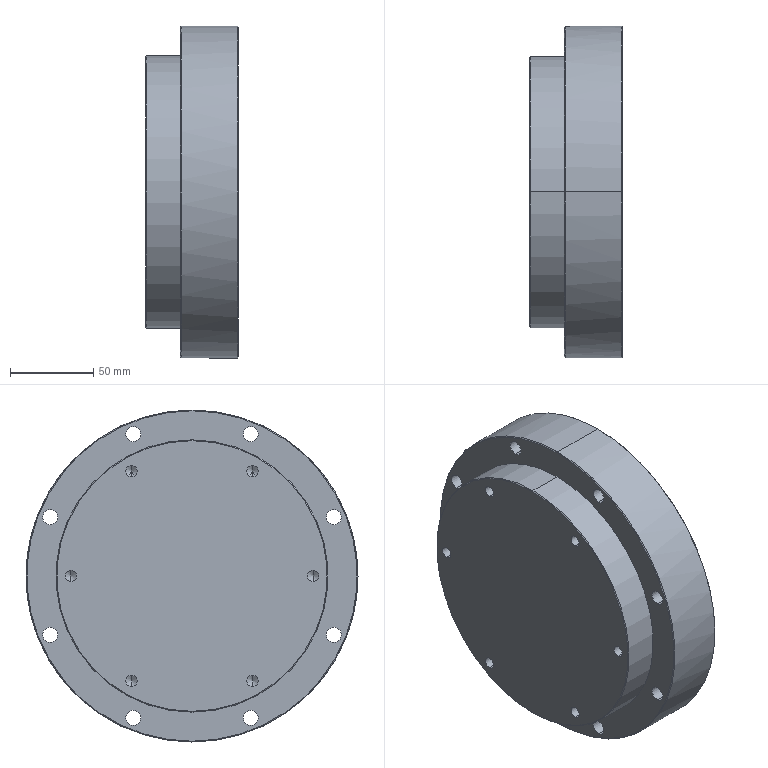Part | SolidWorks | features BaseBody 1 | 1 solid | 53 faces | box 56 x 200 x 200 mm | volume 1520895 mm3 | cylinder 32 | cone 18 | plane 3 | commonest cylinder face diameters 9 x16 6.8 x12 164 x2 200 x2
STEP:
#1=CARTESIAN_POINT('',(56.,85.459,-30.898));
#2=VERTEX_POINT('',#1);
#3=CARTESIAN_POINT('',(56.,85.459,-39.898));
#4=VERTEX_POINT('',#3);
#5=CARTESIAN_POINT('',(56.,85.459,-35.398));
#6=DIRECTION('',(1.,0.,0.));
#7=DIRECTION('',(0.,0.,1.));
#8=AXIS2_PLACEMENT_3D('',#5,#6,#7);
#9=CIRCLE('',#8,4.5);
#10=EDGE_CURVE('',#2,#4,#9,.T.);
#11=ORIENTED_EDGE('',*,*,#10,.T.);
#12=CARTESIAN_POINT('',(21.,85.459,-39.898));
#13=VERTEX_POINT('',#12);
#14=CARTESIAN_POINT('',(56.,85.459,-39.898));
#15=DIRECTION('',(-1.,0.,0.));
#16=VECTOR('',#15,1000.);
#17=LINE('',#14,#16);
#18=EDGE_CURVE('',#4,#13,#17,.T.);
#19=ORIENTED_EDGE('',*,*,#18,.T.);
#20=CARTESIAN_POINT('',(21.,85.459,-30.898));
#21=VERTEX_POINT('',#20);
#22=CARTESIAN_POINT('',(21.,85.459,-35.398));
#23=DIRECTION('',(1.,0.,0.));
#24=DIRECTION('',(0.,0.,1.));
#25=AXIS2_PLACEMENT_3D('',#22,#23,#24);
#26=CIRCLE('',#25,4.5);
#27=EDGE_CURVE('',#21,#13,#26,.T.);
#28=ORIENTED_EDGE('',*,*,#27,.F.);
#29=CARTESIAN_POINT('',(56.,85.459,-30.898));
#30=DIRECTION('',(-1.,0.,0.));
#31=VECTOR('',#30,1000.);
#32=LINE('',#29,#31);
#33=EDGE_CURVE('',#2,#21,#32,.T.);
#34=ORIENTED_EDGE('',*,*,#33,.F.);
#35=EDGE_LOOP('',(#11,#19,#28,#34));
#36=FACE_OUTER_BOUND('',#35,.T.);
#37=CARTESIAN_POINT('',(56.,85.459,-35.398));
#38=DIRECTION('',(-1.,0.,0.));
#39=DIRECTION('',(0.,0.,1.));
#40=AXIS2_PLACEMENT_3D('',#37,#38,#39);
#41=CYLINDRICAL_SURFACE('',#40,4.5);
#42=ADVANCED_FACE('',(#36),#41,.F.);
#43=CARTESIAN_POINT('',(56.,35.398,-80.959));
#44=VERTEX_POINT('',#43);
#45=CARTESIAN_POINT('',(56.,35.398,-89.959));
#46=VERTEX_POINT('',#45);
#47=CARTESIAN_POINT('',(56.,35.398,-85.459));
#48=DIRECTION('',(1.,0.,0.));
#49=DIRECTION('',(0.,0.,1.));
#50=AXIS2_PLACEMENT_3D('',#47,#48,#49);
#51=CIRCLE('',#50,4.5);
#52=EDGE_CURVE('',#44,#46,#51,.T.);
#53=ORIENTED_EDGE('',*,*,#52,.T.);
#54=CARTESIAN_POINT('',(21.,35.398,-89.959));
#55=VERTEX_POINT('',#54);
#56=CARTESIAN_POINT('',(56.,35.398,-89.959));
#57=DIRECTION('',(-1.,0.,0.));
#58=VECTOR('',#57,1000.);
#59=LINE('',#56,#58);
#60=EDGE_CURVE('',#46,#55,#59,.T.);
#61=ORIENTED_EDGE('',*,*,#60,.T.);
#62=CARTESIAN_POINT('',(21.,35.398,-80.959));
#63=VERTEX_POINT('',#62);
#64=CARTESIAN_POINT('',(21.,35.398,-85.459));
#65=DIRECTION('',(1.,0.,0.));
#66=DIRECTION('',(0.,0.,1.));
#67=AXIS2_PLACEMENT_3D('',#64,#65,#66);
#68=CIRCLE('',#67,4.5);
#69=EDGE_CURVE('',#63,#55,#68,.T.);
#70=ORIENTED_EDGE('',*,*,#69,.F.);
#71=CARTESIAN_POINT('',(56.,35.398,-80.959));
#72=DIRECTION('',(-1.,0.,0.));
#73=VECTOR('',#72,1000.);
#74=LINE('',#71,#73);
#75=EDGE_CURVE('',#44,#63,#74,.T.);
#76=ORIENTED_EDGE('',*,*,#75,.F.);
#77=EDGE_LOOP('',(#53,#61,#70,#76));
#78=FACE_OUTER_BOUND('',#77,.T.);
#79=CARTESIAN_POINT('',(56.,35.398,-85.459));
#80=DIRECTION('',(-1.,0.,0.));
#81=DIRECTION('',(0.,0.,1.));
#82=AXIS2_PLACEMENT_3D('',#79,#80,#81);
#83=CYLINDRICAL_SURFACE('',#82,4.5);
#84=ADVANCED_FACE('',(#78),#83,.F.);
#85=CARTESIAN_POINT('',(56.,-35.398,-80.959));
#86=VERTEX_POINT('',#85);
#87=CARTESIAN_POINT('',(56.,-35.398,-89.959));
#88=VERTEX_POINT('',#87);
#89=CARTESIAN_POINT('',(56.,-35.398,-85.459));
#90=DIRECTION('',(1.,0.,0.));
#91=DIRECTION('',(0.,0.,1.));
#92=AXIS2_PLACEMENT_3D('',#89,#90,#91);
#93=CIRCLE('',#92,4.5);
#94=EDGE_CURVE('',#86,#88,#93,.T.);
#95=ORIENTED_EDGE('',*,*,#94,.T.);
#96=CARTESIAN_POINT('',(21.,-35.398,-89.959));
#97=VERTEX_POINT('',#96);
#98=CARTESIAN_POINT('',(56.,-35.398,-89.959));
#99=DIRECTION('',(-1.,0.,0.));
#100=VECTOR('',#99,1000.);
#101=LINE('',#98,#100);
#102=EDGE_CURVE('',#88,#97,#101,.T.);
#103=ORIENTED_EDGE('',*,*,#102,.T.);
#104=CARTESIAN_POINT('',(21.,-35.398,-80.959));
#105=VERTEX_POINT('',#104);
#106=CARTESIAN_POINT('',(21.,-35.398,-85.459));
#107=DIRECTION('',(1.,0.,0.));
#108=DIRECTION('',(0.,0.,1.));
#109=AXIS2_PLACEMENT_3D('',#106,#107,#108);
#110=CIRCLE('',#109,4.5);
#111=EDGE_CURVE('',#105,#97,#110,.T.);
#112=ORIENTED_EDGE('',*,*,#111,.F.);
#113=CARTESIAN_POINT('',(56.,-35.398,-80.959));
#114=DIRECTION('',(-1.,0.,0.));
#115=VECTOR('',#114,1000.);
#116=LINE('',#113,#115);
#117=EDGE_CURVE('',#86,#105,#116,.T.);
#118=ORIENTED_EDGE('',*,*,#117,.F.);
#119=EDGE_LOOP('',(#95,#103,#112,#118));
#120=FACE_OUTER_BOUND('',#119,.T.);
#121=CARTESIAN_POINT('',(56.,-35.398,-85.459));
#122=DIRECTION('',(-1.,0.,0.));
#123=DIRECTION('',(0.,0.,1.));
#124=AXIS2_PLACEMENT_3D('',#121,#122,#123);
#125=CYLINDRICAL_SURFACE('',#124,4.5);
#126=ADVANCED_FACE('',(#120),#125,.F.);
#127=CARTESIAN_POINT('',(56.,-85.459,-30.898));
#128=VERTEX_POINT('',#127);
#129=CARTESIAN_POINT('',(56.,-85.459,-39.898));
#130=VERTEX_POINT('',#129);
#131=CARTESIAN_POINT('',(56.,-85.459,-35.398));
#132=DIRECTION('',(1.,0.,0.));
#133=DIRECTION('',(0.,0.,1.));
#134=AXIS2_PLACEMENT_3D('',#131,#132,#133);
#135=CIRCLE('',#134,4.5);
#136=EDGE_CURVE('',#128,#130,#135,.T.);
#137=ORIENTED_EDGE('',*,*,#136,.T.);
#138=CARTESIAN_POINT('',(21.,-85.459,-39.898));
#139=VERTEX_POINT('',#138);
#140=CARTESIAN_POINT('',(56.,-85.459,-39.898));
#141=DIRECTION('',(-1.,0.,0.));
#142=VECTOR('',#141,1000.);
#143=LINE('',#140,#142);
#144=EDGE_CURVE('',#130,#139,#143,.T.);
#145=ORIENTED_EDGE('',*,*,#144,.T.);
#146=CARTESIAN_POINT('',(21.,-85.459,-30.898));
#147=VERTEX_POINT('',#146);
#148=CARTESIAN_POINT('',(21.,-85.459,-35.398));
#149=DIRECTION('',(1.,0.,0.));
#150=DIRECTION('',(0.,0.,1.));
#151=AXIS2_PLACEMENT_3D('',#148,#149,#150);
#152=CIRCLE('',#151,4.5);
#153=EDGE_CURVE('',#147,#139,#152,.T.);
#154=ORIENTED_EDGE('',*,*,#153,.F.);
#155=CARTESIAN_POINT('',(56.,-85.459,-30.898));
#156=DIRECTION('',(-1.,0.,0.));
#157=VECTOR('',#156,1000.);
#158=LINE('',#155,#157);
#159=EDGE_CURVE('',#128,#147,#158,.T.);
#160=ORIENTED_EDGE('',*,*,#159,.F.);
#161=EDGE_LOOP('',(#137,#145,#154,#160));
#162=FACE_OUTER_BOUND('',#161,.T.);
#163=CARTESIAN_POINT('',(56.,-85.459,-35.398));
#164=DIRECTION('',(-1.,0.,0.));
#165=DIRECTION('',(0.,0.,1.));
#166=AXIS2_PLACEMENT_3D('',#163,#164,#165);
#167=CYLINDRICAL_SURFACE('',#166,4.5);
#168=ADVANCED_FACE('',(#162),#167,.F.);
#169=CARTESIAN_POINT('',(56.,-85.459,39.898));
#170=VERTEX_POINT('',#169);
#171=CARTESIAN_POINT('',(56.,-85.459,30.898));
#172=VERTEX_POINT('',#171);
#173=CARTESIAN_POINT('',(56.,-85.459,35.398));
#174=DIRECTION('',(1.,0.,0.));
#175=DIRECTION('',(0.,0.,1.));
#176=AXIS2_PLACEMENT_3D('',#173,#174,#175);
#177=CIRCLE('',#176,4.5);
#178=EDGE_CURVE('',#170,#172,#177,.T.);
#179=ORIENTED_EDGE('',*,*,#178,.T.);
#180=CARTESIAN_POINT('',(21.,-85.459,30.898));
#181=VERTEX_POINT('',#180);
#182=CARTESIAN_POINT('',(56.,-85.459,30.898));
#183=DIRECTION('',(-1.,0.,0.));
#184=VECTOR('',#183,1000.);
#185=LINE('',#182,#184);
#186=EDGE_CURVE('',#172,#181,#185,.T.);
#187=ORIENTED_EDGE('',*,*,#186,.T.);
#188=CARTESIAN_POINT('',(21.,-85.459,39.898));
#189=VERTEX_POINT('',#188);
#190=CARTESIAN_POINT('',(21.,-85.459,35.398));
#191=DIRECTION('',(1.,0.,0.));
#192=DIRECTION('',(0.,0.,1.));
#193=AXIS2_PLACEMENT_3D('',#190,#191,#192);
#194=CIRCLE('',#193,4.5);
#195=EDGE_CURVE('',#189,#181,#194,.T.);
#196=ORIENTED_EDGE('',*,*,#195,.F.);
#197=CARTESIAN_POINT('',(56.,-85.459,39.898));
#198=DIRECTION('',(-1.,0.,0.));
#199=VECTOR('',#198,1000.);
#200=LINE('',#197,#199);
#201=EDGE_CURVE('',#170,#189,#200,.T.);
#202=ORIENTED_EDGE('',*,*,#201,.F.);
#203=EDGE_LOOP('',(#179,#187,#196,#202));
#204=FACE_OUTER_BOUND('',#203,.T.);
#205=CARTESIAN_POINT('',(56.,-85.459,35.398));
#206=DIRECTION('',(-1.,0.,0.));
#207=DIRECTION('',(0.,0.,1.));
#208=AXIS2_PLACEMENT_3D('',#205,#206,#207);
#209=CYLINDRICAL_SURFACE('',#208,4.5);
#210=ADVANCED_FACE('',(#204),#209,.F.);
#211=CARTESIAN_POINT('',(56.,-35.398,89.959));
#212=VERTEX_POINT('',#211);
#213=CARTESIAN_POINT('',(56.,-35.398,80.959));
#214=VERTEX_POINT('',#213);
#215=CARTESIAN_POINT('',(56.,-35.398,85.459));
#216=DIRECTION('',(1.,0.,0.));
#217=DIRECTION('',(0.,0.,1.));
#218=AXIS2_PLACEMENT_3D('',#215,#216,#217);
#219=CIRCLE('',#218,4.5);
#220=EDGE_CURVE('',#212,#214,#219,.T.);
#221=ORIENTED_EDGE('',*,*,#220,.T.);
#222=CARTESIAN_POINT('',(21.,-35.398,80.959));
#223=VERTEX_POINT('',#222);
#224=CARTESIAN_POINT('',(56.,-35.398,80.959));
#225=DIRECTION('',(-1.,0.,0.));
#226=VECTOR('',#225,1000.);
#227=LINE('',#224,#226);
#228=EDGE_CURVE('',#214,#223,#227,.T.);
#229=ORIENTED_EDGE('',*,*,#228,.T.);
#230=CARTESIAN_POINT('',(21.,-35.398,89.959));
#231=VERTEX_POINT('',#230);
#232=CARTESIAN_POINT('',(21.,-35.398,85.459));
#233=DIRECTION('',(1.,0.,0.));
#234=DIRECTION('',(0.,0.,1.));
#235=AXIS2_PLACEMENT_3D('',#232,#233,#234);
#236=CIRCLE('',#235,4.5);
#237=EDGE_CURVE('',#231,#223,#236,.T.);
#238=ORIENTED_EDGE('',*,*,#237,.F.);
#239=CARTESIAN_POINT('',(56.,-35.398,89.959));
#240=DIRECTION('',(-1.,0.,0.));
#241=VECTOR('',#240,1000.);
#242=LINE('',#239,#241);
#243=EDGE_CURVE('',#212,#231,#242,.T.);
#244=ORIENTED_EDGE('',*,*,#243,.F.);
#245=EDGE_LOOP('',(#221,#229,#238,#244));
#246=FACE_OUTER_BOUND('',#245,.T.);
#247=CARTESIAN_POINT('',(56.,-35.398,85.459));
#248=DIRECTION('',(-1.,0.,0.));
#249=DIRECTION('',(0.,0.,1.));
#250=AXIS2_PLACEMENT_3D('',#247,#248,#249);
#251=CYLINDRICAL_SURFACE('',#250,4.5);
#252=ADVANCED_FACE('',(#246),#251,.F.);
#253=CARTESIAN_POINT('',(56.,35.398,89.959));
#254=VERTEX_POINT('',#253);
#255=CARTESIAN_POINT('',(56.,35.398,80.959));
#256=VERTEX_POINT('',#255);
#257=CARTESIAN_POINT('',(56.,35.398,85.459));
#258=DIRECTION('',(1.,0.,0.));
#259=DIRECTION('',(0.,0.,1.));
#260=AXIS2_PLACEMENT_3D('',#257,#258,#259);
#261=CIRCLE('',#260,4.5);
#262=EDGE_CURVE('',#254,#256,#261,.T.);
#263=ORIENTED_EDGE('',*,*,#262,.T.);
#264=CARTESIAN_POINT('',(21.,35.398,80.959));
#265=VERTEX_POINT('',#264);
#266=CARTESIAN_POINT('',(56.,35.398,80.959));
#267=DIRECTION('',(-1.,0.,0.));
#268=VECTOR('',#267,1000.);
#269=LINE('',#266,#268);
#270=EDGE_CURVE('',#256,#265,#269,.T.);
#271=ORIENTED_EDGE('',*,*,#270,.T.);
#272=CARTESIAN_POINT('',(21.,35.398,89.959));
#273=VERTEX_POINT('',#272);
#274=CARTESIAN_POINT('',(21.,35.398,85.459));
#275=DIRECTION('',(1.,0.,0.));
#276=DIRECTION('',(0.,0.,1.));
#277=AXIS2_PLACEMENT_3D('',#274,#275,#276);
#278=CIRCLE('',#277,4.5);
#279=EDGE_CURVE('',#273,#265,#278,.T.);
#280=ORIENTED_EDGE('',*,*,#279,.F.);
#281=CARTESIAN_POINT('',(56.,35.398,89.959));
#282=DIRECTION('',(-1.,0.,0.));
#283=VECTOR('',#282,1000.);
#284=LINE('',#281,#283);
#285=EDGE_CURVE('',#254,#273,#284,.T.);
#286=ORIENTED_EDGE('',*,*,#285,.F.);
#287=EDGE_LOOP('',(#263,#271,#280,#286));
#288=FACE_OUTER_BOUND('',#287,.T.);
#289=CARTESIAN_POINT('',(56.,35.398,85.459));
#290=DIRECTION('',(-1.,0.,0.));
#291=DIRECTION('',(0.,0.,1.));
#292=AXIS2_PLACEMENT_3D('',#289,#290,#291);
#293=CYLINDRICAL_SURFACE('',#292,4.5);
#294=ADVANCED_FACE('',(#288),#293,.F.);
#295=CARTESIAN_POINT('',(56.,85.459,39.898));
#296=VERTEX_POINT('',#295);
#297=CARTESIAN_POINT('',(56.,85.459,30.898));
#298=VERTEX_POINT('',#297);
#299=CARTESIAN_POINT('',(56.,85.459,35.398));
#300=DIRECTION('',(1.,0.,0.));
#301=DIRECTION('',(0.,0.,1.));
#302=AXIS2_PLACEMENT_3D('',#299,#300,#301);
#303=CIRCLE('',#302,4.5);
#304=EDGE_CURVE('',#296,#298,#303,.T.);
#305=ORIENTED_EDGE('',*,*,#304,.T.);
#306=CARTESIAN_POINT('',(21.,85.459,30.898));
#307=VERTEX_POINT('',#306);
#308=CARTESIAN_POINT('',(56.,85.459,30.898));
#309=DIRECTION('',(-1.,0.,0.));
#310=VECTOR('',#309,1000.);
#311=LINE('',#308,#310);
#312=EDGE_CURVE('',#298,#307,#311,.T.);
#313=ORIENTED_EDGE('',*,*,#312,.T.);
#314=CARTESIAN_POINT('',(21.,85.459,39.898));
#315=VERTEX_POINT('',#314);
#316=CARTESIAN_POINT('',(21.,85.459,35.398));
#317=DIRECTION('',(1.,0.,0.));
#318=DIRECTION('',(0.,0.,1.));
#319=AXIS2_PLACEMENT_3D('',#316,#317,#318);
#320=CIRCLE('',#319,4.5);
#321=EDGE_CURVE('',#315,#307,#320,.T.);
#322=ORIENTED_EDGE('',*,*,#321,.F.);
#323=CARTESIAN_POINT('',(56.,85.459,39.898));
#324=DIRECTION('',(-1.,0.,0.));
#325=VECTOR('',#324,1000.);
#326=LINE('',#323,#325);
#327=EDGE_CURVE('',#296,#315,#326,.T.);
#328=ORIENTED_EDGE('',*,*,#327,.F.);
#329=EDGE_LOOP('',(#305,#313,#322,#328));
#330=FACE_OUTER_BOUND('',#329,.T.);
#331=CARTESIAN_POINT('',(56.,85.459,35.398));
#332=DIRECTION('',(-1.,0.,0.));
#333=DIRECTION('',(0.,0.,1.));
#334=AXIS2_PLACEMENT_3D('',#331,#332,#333);
#335=CYLINDRICAL_SURFACE('',#334,4.5);
#336=ADVANCED_FACE('',(#330),#335,.F.);
#337=CARTESIAN_POINT('',(56.,-99.5,0.));
#338=VERTEX_POINT('',#337);
#339=CARTESIAN_POINT('',(56.,99.5,0.));
#340=VERTEX_POINT('',#339);
#341=CARTESIAN_POINT('',(56.,0.,0.));
#342=DIRECTION('',(-1.,0.,0.));
#343=DIRECTION('',(0.,-1.,0.));
#344=AXIS2_PLACEMENT_3D('',#341,#342,#343);
#345=CIRCLE('',#344,99.5);
#346=EDGE_CURVE('',#338,#340,#345,.T.);
#347=ORIENTED_EDGE('',*,*,#346,.T.);
#348=CARTESIAN_POINT('',(55.5,100.,0.));
#349=VERTEX_POINT('',#348);
#350=CARTESIAN_POINT('',(55.5,100.,0.));
#351=DIRECTION('',(-0.7071,0.7071,0.));
#352=VECTOR('',#351,1000.);
#353=LINE('',#350,#352);
#354=EDGE_CURVE('',#340,#349,#353,.T.);
#355=ORIENTED_EDGE('',*,*,#354,.T.);
#356=CARTESIAN_POINT('',(55.5,0.,100.));
#357=VERTEX_POINT('',#356);
#358=CARTESIAN_POINT('',(55.5,0.,0.));
#359=DIRECTION('',(1.,0.,0.));
#360=DIRECTION('',(0.,0.,1.));
#361=AXIS2_PLACEMENT_3D('',#358,#359,#360);
#362=CIRCLE('',#361,100.);
#363=EDGE_CURVE('',#349,#357,#362,.T.);
#364=ORIENTED_EDGE('',*,*,#363,.T.);
#365=CARTESIAN_POINT('',(55.5,-100.,0.));
#366=VERTEX_POINT('',#365);
#367=CARTESIAN_POINT('',(55.5,0.,0.));
#368=DIRECTION('',(1.,0.,0.));
#369=DIRECTION('',(0.,0.,1.));
#370=AXIS2_PLACEMENT_3D('',#367,#368,#369);
#371=CIRCLE('',#370,100.);
#372=EDGE_CURVE('',#357,#366,#371,.T.);
#373=ORIENTED_EDGE('',*,*,#372,.T.);
#374=CARTESIAN_POINT('',(55.5,-100.,0.));
#375=DIRECTION('',(-0.7071,-0.7071,0.));
#376=VECTOR('',#375,1000.);
#377=LINE('',#374,#376);
#378=EDGE_CURVE('',#338,#366,#377,.T.);
#379=ORIENTED_EDGE('',*,*,#378,.F.);
#380=EDGE_LOOP('',(#347,#355,#364,#373,#379));
#381=FACE_OUTER_BOUND('',#380,.T.);
#382=CARTESIAN_POINT('',(55.5,0.,0.));
#383=DIRECTION('',(-1.,0.,0.));
#384=DIRECTION('',(0.,-1.,0.));
#385=AXIS2_PLACEMENT_3D('',#382,#383,#384);
#386=CONICAL_SURFACE('',#385,100.,0.7854);
#387=ADVANCED_FACE('',(#381),#386,.T.);
#388=CARTESIAN_POINT('',(55.5,0.,-100.));
#389=VERTEX_POINT('',#388);
#390=CARTESIAN_POINT('',(55.5,0.,0.));
#391=DIRECTION('',(1.,0.,0.));
#392=DIRECTION('',(0.,0.,1.));
#393=AXIS2_PLACEMENT_3D('',#390,#391,#392);
#394=CIRCLE('',#393,100.);
#395=EDGE_CURVE('',#389,#349,#394,.T.);
#396=ORIENTED_EDGE('',*,*,#395,.F.);
#397=CARTESIAN_POINT('',(21.5,0.,-100.));
#398=VERTEX_POINT('',#397);
#399=CARTESIAN_POINT('',(0.,0.,-100.));
#400=DIRECTION('',(-1.,0.,0.));
#401=VECTOR('',#400,1000.);
#402=LINE('',#399,#401);
#403=EDGE_CURVE('',#389,#398,#402,.T.);
#404=ORIENTED_EDGE('',*,*,#403,.T.);
#405=CARTESIAN_POINT('',(21.5,0.,100.));
#406=VERTEX_POINT('',#405);
#407=CARTESIAN_POINT('',(21.5,0.,0.));
#408=DIRECTION('',(1.,0.,0.));
#409=DIRECTION('',(0.,0.,1.));
#410=AXIS2_PLACEMENT_3D('',#407,#408,#409);
#411=CIRCLE('',#410,100.);
#412=EDGE_CURVE('',#398,#406,#411,.T.);
#413=ORIENTED_EDGE('',*,*,#412,.T.);
#414=CARTESIAN_POINT('',(0.,0.,100.));
#415=DIRECTION('',(-1.,0.,0.));
#416=VECTOR('',#415,1000.);
#417=LINE('',#414,#416);
#418=EDGE_CURVE('',#357,#406,#417,.T.);
#419=ORIENTED_EDGE('',*,*,#418,.F.);
#420=ORIENTED_EDGE('',*,*,#363,.F.);
#421=EDGE_LOOP('',(#396,#404,#413,#419,#420));
#422=FACE_OUTER_BOUND('',#421,.T.);
#423=CARTESIAN_POINT('',(0.,0.,0.));
#424=DIRECTION('',(-1.,0.,0.));
#425=DIRECTION('',(0.,0.,1.));
#426=AXIS2_PLACEMENT_3D('',#423,#424,#425);
#427=CYLINDRICAL_SURFACE('',#426,100.);
#428=ADVANCED_FACE('',(#422),#427,.T.);
#429=CARTESIAN_POINT('',(21.,0.,82.));
#430=VERTEX_POINT('',#429);
#431=CARTESIAN_POINT('',(21.,0.,-82.));
#432=VERTEX_POINT('',#431);
#433=CARTESIAN_POINT('',(21.,0.,0.));
#434=DIRECTION('',(-1.,0.,0.));
#435=DIRECTION('',(0.,0.,1.));
#436=AXIS2_PLACEMENT_3D('',#433,#434,#435);
#437=CIRCLE('',#436,82.);
#438=EDGE_CURVE('',#430,#432,#437,.T.);
#439=ORIENTED_EDGE('',*,*,#438,.T.);
#440=CARTESIAN_POINT('',(0.5,0.,-82.));
#441=VERTEX_POINT('',#440);
#442=CARTESIAN_POINT('',(0.,0.,-82.));
#443=DIRECTION('',(-1.,0.,0.));
#444=VECTOR('',#443,1000.);
#445=LINE('',#442,#444);
#446=EDGE_CURVE('',#432,#441,#445,.T.);
#447=ORIENTED_EDGE('',*,*,#446,.T.);
#448=CARTESIAN_POINT('',(0.5,0.,82.));
#449=VERTEX_POINT('',#448);
#450=CARTESIAN_POINT('',(0.5,0.,0.));
#451=DIRECTION('',(1.,0.,0.));
#452=DIRECTION('',(0.,0.,1.));
#453=AXIS2_PLACEMENT_3D('',#450,#451,#452);
#454=CIRCLE('',#453,82.);
#455=EDGE_CURVE('',#441,#449,#454,.T.);
#456=ORIENTED_EDGE('',*,*,#455,.T.);
#457=CARTESIAN_POINT('',(0.,0.,82.));
#458=DIRECTION('',(-1.,0.,0.));
#459=VECTOR('',#458,1000.);
#460=LINE('',#457,#459);
#461=EDGE_CURVE('',#430,#449,#460,.T.);
#462=ORIENTED_EDGE('',*,*,#461,.F.);
#463=EDGE_LOOP('',(#439,#447,#456,#462));
#464=FACE_OUTER_BOUND('',#463,.T.);
#465=CARTESIAN_POINT('',(0.,0.,0.));
#466=DIRECTION('',(-1.,0.,0.));
#467=DIRECTION('',(0.,0.,1.));
#468=AXIS2_PLACEMENT_3D('',#465,#466,#467);
#469=CYLINDRICAL_SURFACE('',#468,82.);
#470=ADVANCED_FACE('',(#464),#469,.T.);
#471=CARTESIAN_POINT('',(21.,0.,-99.5));
#472=VERTEX_POINT('',#471);
#473=CARTESIAN_POINT('',(21.,0.,99.5));
#474=VERTEX_POINT('',#473);
#475=CARTESIAN_POINT('',(21.,0.,0.));
#476=DIRECTION('',(1.,0.,0.));
#477=DIRECTION('',(0.,0.,-1.));
#478=AXIS2_PLACEMENT_3D('',#475,#476,#477);
#479=CIRCLE('',#478,99.5);
#480=EDGE_CURVE('',#472,#474,#479,.T.);
#481=ORIENTED_EDGE('',*,*,#480,.T.);
#482=CARTESIAN_POINT('',(21.5,0.,100.));
#483=DIRECTION('',(0.7071,0.,0.7071));
#484=VECTOR('',#483,1000.);
#485=LINE('',#482,#484);
#486=EDGE_CURVE('',#474,#406,#485,.T.);
#487=ORIENTED_EDGE('',*,*,#486,.T.);
#488=ORIENTED_EDGE('',*,*,#412,.F.);
#489=CARTESIAN_POINT('',(21.5,0.,-100.));
#490=DIRECTION('',(0.7071,0.,-0.7071));
#491=VECTOR('',#490,1000.);
#492=LINE('',#489,#491);
#493=EDGE_CURVE('',#472,#398,#492,.T.);
#494=ORIENTED_EDGE('',*,*,#493,.F.);
#495=EDGE_LOOP('',(#481,#487,#488,#494));
#496=FACE_OUTER_BOUND('',#495,.T.);
#497=CARTESIAN_POINT('',(21.5,0.,0.));
#498=DIRECTION('',(1.,0.,0.));
#499=DIRECTION('',(0.,0.,-1.));
#500=AXIS2_PLACEMENT_3D('',#497,#498,#499);
#501=CONICAL_SURFACE('',#500,100.,0.7854);
#502=ADVANCED_FACE('',(#496),#501,.T.);
#503=CARTESIAN_POINT('',(0.,0.,-81.5));
#504=VERTEX_POINT('',#503);
#505=CARTESIAN_POINT('',(0.,0.,81.5));
#506=VERTEX_POINT('',#505);
#507=CARTESIAN_POINT('',(0.,0.,0.));
#508=DIRECTION('',(1.,0.,0.));
#509=DIRECTION('',(0.,0.,-1.));
#510=AXIS2_PLACEMENT_3D('',#507,#508,#509);
#511=CIRCLE('',#510,81.5);
#512=EDGE_CURVE('',#504,#506,#511,.T.);
#513=ORIENTED_EDGE('',*,*,#512,.T.);
#514=CARTESIAN_POINT('',(0.5,0.,82.));
#515=DIRECTION('',(0.7071,0.,0.7071));
#516=VECTOR('',#515,1000.);
#517=LINE('',#514,#516);
#518=EDGE_CURVE('',#506,#449,#517,.T.);
#519=ORIENTED_EDGE('',*,*,#518,.T.);
#520=ORIENTED_EDGE('',*,*,#455,.F.);
#521=CARTESIAN_POINT('',(0.5,0.,-82.));
#522=DIRECTION('',(0.7071,0.,-0.7071));
#523=VECTOR('',#522,1000.);
#524=LINE('',#521,#523);
#525=EDGE_CURVE('',#504,#441,#524,.T.);
#526=ORIENTED_EDGE('',*,*,#525,.F.);
#527=EDGE_LOOP('',(#513,#519,#520,#526));
#528=FACE_OUTER_BOUND('',#527,.T.);
#529=CARTESIAN_POINT('',(0.5,0.,0.));
#530=DIRECTION('',(1.,0.,0.));
#531=DIRECTION('',(0.,0.,-1.));
#532=AXIS2_PLACEMENT_3D('',#529,#530,#531);
#533=CONICAL_SURFACE('',#532,82.,0.7854);
#534=ADVANCED_FACE('',(#528),#533,.T.);
#535=CARTESIAN_POINT('',(18.75,73.,-3.4));
#536=VERTEX_POINT('',#535);
#537=CARTESIAN_POINT('',(18.75,73.,3.4));
#538=VERTEX_POINT('',#537);
#539=CARTESIAN_POINT('',(18.75,73.,0.));
#540=DIRECTION('',(-1.,0.,0.));
#541=DIRECTION('',(0.,0.,1.));
#542=AXIS2_PLACEMENT_3D('',#539,#540,#541);
#543=CIRCLE('',#542,3.4);
#544=EDGE_CURVE('',#536,#538,#543,.T.);
#545=ORIENTED_EDGE('',*,*,#544,.F.);
#546=CARTESIAN_POINT('',(0.,73.,-3.4));
#547=VERTEX_POINT('',#546);
#548=CARTESIAN_POINT('',(0.,73.,-3.4));
#549=DIRECTION('',(-1.,0.,0.));
#550=VECTOR('',#549,1000.);
#551=LINE('',#548,#550);
#552=EDGE_CURVE('',#536,#547,#551,.T.);
#553=ORIENTED_EDGE('',*,*,#552,.T.);
#554=CARTESIAN_POINT('',(0.,73.,3.4));
#555=VERTEX_POINT('',#554);
#556=CARTESIAN_POINT('',(0.,73.,0.));
#557=DIRECTION('',(-1.,0.,0.));
#558=DIRECTION('',(0.,0.,1.));
#559=AXIS2_PLACEMENT_3D('',#556,#557,#558);
#560=CIRCLE('',#559,3.4);
#561=EDGE_CURVE('',#547,#555,#560,.T.);
#562=ORIENTED_EDGE('',*,*,#561,.T.);
#563=CARTESIAN_POINT('',(0.,73.,3.4));
#564=DIRECTION('',(-1.,0.,0.));
#565=VECTOR('',#564,1000.);
#566=LINE('',#563,#565);
#567=EDGE_CURVE('',#538,#555,#566,.T.);
#568=ORIENTED_EDGE('',*,*,#567,.F.);
#569=EDGE_LOOP('',(#545,#553,#562,#568));
#570=FACE_OUTER_BOUND('',#569,.T.);
#571=CARTESIAN_POINT('',(0.,73.,0.));
#572=DIRECTION('',(-1.,0.,0.));
#573=DIRECTION('',(0.,0.,1.));
#574=AXIS2_PLACEMENT_3D('',#571,#572,#573);
#575=CYLINDRICAL_SURFACE('',#574,3.4);
#576=ADVANCED_FACE('',(#570),#575,.F.);
#577=CARTESIAN_POINT('',(18.75,36.5,-66.62));
#578=VERTEX_POINT('',#577);
#579=CARTESIAN_POINT('',(18.75,36.5,-59.82));
#580=VERTEX_POINT('',#579);
#581=CARTESIAN_POINT('',(18.75,36.5,-63.22));
#582=DIRECTION('',(-1.,0.,0.));
#583=DIRECTION('',(0.,0.,1.));
#584=AXIS2_PLACEMENT_3D('',#581,#582,#583);
#585=CIRCLE('',#584,3.4);
#586=EDGE_CURVE('',#578,#580,#585,.T.);
#587=ORIENTED_EDGE('',*,*,#586,.F.);
#588=CARTESIAN_POINT('',(0.,36.5,-66.62));
#589=VERTEX_POINT('',#588);
#590=CARTESIAN_POINT('',(0.,36.5,-66.62));
#591=DIRECTION('',(-1.,0.,0.));
#592=VECTOR('',#591,1000.);
#593=LINE('',#590,#592);
#594=EDGE_CURVE('',#578,#589,#593,.T.);
#595=ORIENTED_EDGE('',*,*,#594,.T.);
#596=CARTESIAN_POINT('',(0.,36.5,-59.82));
#597=VERTEX_POINT('',#596);
#598=CARTESIAN_POINT('',(0.,36.5,-63.22));
#599=DIRECTION('',(-1.,0.,0.));
#600=DIRECTION('',(0.,0.,1.));
#601=AXIS2_PLACEMENT_3D('',#598,#599,#600);
#602=CIRCLE('',#601,3.4);
#603=EDGE_CURVE('',#589,#597,#602,.T.);
#604=ORIENTED_EDGE('',*,*,#603,.T.);
#605=CARTESIAN_POINT('',(0.,36.5,-59.82));
#606=DIRECTION('',(-1.,0.,0.));
#607=VECTOR('',#606,1000.);
#608=LINE('',#605,#607);
#609=EDGE_CURVE('',#580,#597,#608,.T.);
#610=ORIENTED_EDGE('',*,*,#609,.F.);
#611=EDGE_LOOP('',(#587,#595,#604,#610));
#612=FACE_OUTER_BOUND('',#611,.T.);
#613=CARTESIAN_POINT('',(0.,36.5,-63.22));
#614=DIRECTION('',(-1.,0.,0.));
#615=DIRECTION('',(0.,0.,1.));
#616=AXIS2_PLACEMENT_3D('',#613,#614,#615);
#617=CYLINDRICAL_SURFACE('',#616,3.4);
#618=ADVANCED_FACE('',(#612),#617,.F.);
#619=CARTESIAN_POINT('',(18.75,-36.5,-66.62));
#620=VERTEX_POINT('',#619);
#621=CARTESIAN_POINT('',(18.75,-36.5,-59.82));
#622=VERTEX_POINT('',#621);
#623=CARTESIAN_POINT('',(18.75,-36.5,-63.22));
#624=DIRECTION('',(-1.,0.,0.));
#625=DIRECTION('',(0.,0.,1.));
#626=AXIS2_PLACEMENT_3D('',#623,#624,#625);
#627=CIRCLE('',#626,3.4);
#628=EDGE_CURVE('',#620,#622,#627,.T.);
#629=ORIENTED_EDGE('',*,*,#628,.F.);
#630=CARTESIAN_POINT('',(0.,-36.5,-66.62));
#631=VERTEX_POINT('',#630);
#632=CARTESIAN_POINT('',(0.,-36.5,-66.62));
#633=DIRECTION('',(-1.,0.,0.));
#634=VECTOR('',#633,1000.);
#635=LINE('',#632,#634);
#636=EDGE_CURVE('',#620,#631,#635,.T.);
#637=ORIENTED_EDGE('',*,*,#636,.T.);
#638=CARTESIAN_POINT('',(0.,-36.5,-59.82));
#639=VERTEX_POINT('',#638);
#640=CARTESIAN_POINT('',(0.,-36.5,-63.22));
#641=DIRECTION('',(-1.,0.,0.));
#642=DIRECTION('',(0.,0.,1.));
#643=AXIS2_PLACEMENT_3D('',#640,#641,#642);
#644=CIRCLE('',#643,3.4);
#645=EDGE_CURVE('',#631,#639,#644,.T.);
#646=ORIENTED_EDGE('',*,*,#645,.T.);
#647=CARTESIAN_POINT('',(0.,-36.5,-59.82));
#648=DIRECTION('',(-1.,0.,0.));
#649=VECTOR('',#648,1000.);
#650=LINE('',#647,#649);
#651=EDGE_CURVE('',#622,#639,#650,.T.);
#652=ORIENTED_EDGE('',*,*,#651,.F.);
#653=EDGE_LOOP('',(#629,#637,#646,#652));
#654=FACE_OUTER_BOUND('',#653,.T.);
#655=CARTESIAN_POINT('',(0.,-36.5,-63.22));
#656=DIRECTION('',(-1.,0.,0.));
#657=DIRECTION('',(0.,0.,1.));
#658=AXIS2_PLACEMENT_3D('',#655,#656,#657);
#659=CYLINDRICAL_SURFACE('',#658,3.4);
#660=ADVANCED_FACE('',(#654),#659,.F.);
#661=CARTESIAN_POINT('',(18.75,-73.,-3.4));
#662=VERTEX_POINT('',#661);
#663=CARTESIAN_POINT('',(18.75,-73.,3.4));
#664=VERTEX_POINT('',#663);
#665=CARTESIAN_POINT('',(18.75,-73.,0.));
#666=DIRECTION('',(-1.,0.,0.));
#667=DIRECTION('',(0.,0.,1.));
#668=AXIS2_PLACEMENT_3D('',#665,#666,#667);
#669=CIRCLE('',#668,3.4);
#670=EDGE_CURVE('',#662,#664,#669,.T.);
#671=ORIENTED_EDGE('',*,*,#670,.F.);
#672=CARTESIAN_POINT('',(0.,-73.,-3.4));
#673=VERTEX_POINT('',#672);
#674=CARTESIAN_POINT('',(0.,-73.,-3.4));
#675=DIRECTION('',(-1.,0.,0.));
#676=VECTOR('',#675,1000.);
#677=LINE('',#674,#676);
#678=EDGE_CURVE('',#662,#673,#677,.T.);
#679=ORIENTED_EDGE('',*,*,#678,.T.);
#680=CARTESIAN_POINT('',(0.,-73.,3.4));
#681=VERTEX_POINT('',#680);
#682=CARTESIAN_POINT('',(0.,-73.,0.));
#683=DIRECTION('',(-1.,0.,0.));
#684=DIRECTION('',(0.,0.,1.));
#685=AXIS2_PLACEMENT_3D('',#682,#683,#684);
#686=CIRCLE('',#685,3.4);
#687=EDGE_CURVE('',#673,#681,#686,.T.);
#688=ORIENTED_EDGE('',*,*,#687,.T.);
#689=CARTESIAN_POINT('',(0.,-73.,3.4));
#690=DIRECTION('',(-1.,0.,0.));
#691=VECTOR('',#690,1000.);
#692=LINE('',#689,#691);
#693=EDGE_CURVE('',#664,#681,#692,.T.);
#694=ORIENTED_EDGE('',*,*,#693,.F.);
#695=EDGE_LOOP('',(#671,#679,#688,#694));
#696=FACE_OUTER_BOUND('',#695,.T.);
#697=CARTESIAN_POINT('',(0.,-73.,0.));
#698=DIRECTION('',(-1.,0.,0.));
#699=DIRECTION('',(0.,0.,1.));
#700=AXIS2_PLACEMENT_3D('',#697,#698,#699);
#701=CYLINDRICAL_SURFACE('',#700,3.4);
#702=ADVANCED_FACE('',(#696),#701,.F.);
#703=CARTESIAN_POINT('',(18.75,-36.5,59.82));
#704=VERTEX_POINT('',#703);
#705=CARTESIAN_POINT('',(18.75,-36.5,66.62));
#706=VERTEX_POINT('',#705);
#707=CARTESIAN_POINT('',(18.75,-36.5,63.22));
#708=DIRECTION('',(-1.,0.,0.));
#709=DIRECTION('',(0.,0.,1.));
#710=AXIS2_PLACEMENT_3D('',#707,#708,#709);
#711=CIRCLE('',#710,3.4);
#712=EDGE_CURVE('',#704,#706,#711,.T.);
#713=ORIENTED_EDGE('',*,*,#712,.F.);
#714=CARTESIAN_POINT('',(0.,-36.5,59.82));
#715=VERTEX_POINT('',#714);
#716=CARTESIAN_POINT('',(0.,-36.5,59.82));
#717=DIRECTION('',(-1.,0.,0.));
#718=VECTOR('',#717,1000.);
#719=LINE('',#716,#718);
#720=EDGE_CURVE('',#704,#715,#719,.T.);
#721=ORIENTED_EDGE('',*,*,#720,.T.);
#722=CARTESIAN_POINT('',(0.,-36.5,66.62));
#723=VERTEX_POINT('',#722);
#724=CARTESIAN_POINT('',(0.,-36.5,63.22));
#725=DIRECTION('',(-1.,0.,0.));
#726=DIRECTION('',(0.,0.,1.));
#727=AXIS2_PLACEMENT_3D('',#724,#725,#726);
#728=CIRCLE('',#727,3.4);
#729=EDGE_CURVE('',#715,#723,#728,.T.);
#730=ORIENTED_EDGE('',*,*,#729,.T.);
#731=CARTESIAN_POINT('',(0.,-36.5,66.62));
#732=DIRECTION('',(-1.,0.,0.));
#733=VECTOR('',#732,1000.);
#734=LINE('',#731,#733);
#735=EDGE_CURVE('',#706,#723,#734,.T.);
#736=ORIENTED_EDGE('',*,*,#735,.F.);
#737=EDGE_LOOP('',(#713,#721,#730,#736));
#738=FACE_OUTER_BOUND('',#737,.T.);
#739=CARTESIAN_POINT('',(0.,-36.5,63.22));
#740=DIRECTION('',(-1.,0.,0.));
#741=DIRECTION('',(0.,0.,1.));
#742=AXIS2_PLACEMENT_3D('',#739,#740,#741);
#743=CYLINDRICAL_SURFACE('',#742,3.4);
#744=ADVANCED_FACE('',(#738),#743,.F.);
#745=CARTESIAN_POINT('',(18.75,36.5,59.82));
#746=VERTEX_POINT('',#745);
#747=CARTESIAN_POINT('',(18.75,36.5,66.62));
#748=VERTEX_POINT('',#747);
#749=CARTESIAN_POINT('',(18.75,36.5,63.22));
#750=DIRECTION('',(-1.,0.,0.));
#751=DIRECTION('',(0.,0.,1.));
#752=AXIS2_PLACEMENT_3D('',#749,#750,#751);
#753=CIRCLE('',#752,3.4);
#754=EDGE_CURVE('',#746,#748,#753,.T.);
#755=ORIENTED_EDGE('',*,*,#754,.F.);
#756=CARTESIAN_POINT('',(0.,36.5,59.82));
#757=VERTEX_POINT('',#756);
#758=CARTESIAN_POINT('',(0.,36.5,59.82));
#759=DIRECTION('',(-1.,0.,0.));
#760=VECTOR('',#759,1000.);
#761=LINE('',#758,#760);
#762=EDGE_CURVE('',#746,#757,#761,.T.);
#763=ORIENTED_EDGE('',*,*,#762,.T.);
#764=CARTESIAN_POINT('',(0.,36.5,66.62));
#765=VERTEX_POINT('',#764);
#766=CARTESIAN_POINT('',(0.,36.5,63.22));
#767=DIRECTION('',(-1.,0.,0.));
#768=DIRECTION('',(0.,0.,1.));
#769=AXIS2_PLACEMENT_3D('',#766,#767,#768);
#770=CIRCLE('',#769,3.4);
#771=EDGE_CURVE('',#757,#765,#770,.T.);
#772=ORIENTED_EDGE('',*,*,#771,.T.);
#773=CARTESIAN_POINT('',(0.,36.5,66.62));
#774=DIRECTION('',(-1.,0.,0.));
#775=VECTOR('',#774,1000.);
#776=LINE('',#773,#775);
#777=EDGE_CURVE('',#748,#765,#776,.T.);
#778=ORIENTED_EDGE('',*,*,#777,.F.);
#779=EDGE_LOOP('',(#755,#763,#772,#778));
#780=FACE_OUTER_BOUND('',#779,.T.);
#781=CARTESIAN_POINT('',(0.,36.5,63.22));
#782=DIRECTION('',(-1.,0.,0.));
#783=DIRECTION('',(0.,0.,1.));
#784=AXIS2_PLACEMENT_3D('',#781,#782,#783);
#785=CYLINDRICAL_SURFACE('',#784,3.4);
#786=ADVANCED_FACE('',(#780),#785,.F.);
#787=CARTESIAN_POINT('',(20.793,73.,0.));
#788=VERTEX_POINT('',#787);
#789=CARTESIAN_POINT('',(18.75,73.,3.4));
#790=DIRECTION('',(-0.515,0.,0.8572));
#791=VECTOR('',#790,1000.);
#792=LINE('',#789,#791);
#793=EDGE_CURVE('',#788,#538,#792,.T.);
#794=ORIENTED_EDGE('',*,*,#793,.F.);
#795=CARTESIAN_POINT('',(18.75,73.,-3.4));
#796=DIRECTION('',(-0.515,0.,-0.8572));
#797=VECTOR('',#796,1000.);
#798=LINE('',#795,#797);
#799=EDGE_CURVE('',#788,#536,#798,.T.);
#800=ORIENTED_EDGE('',*,*,#799,.T.);
#801=ORIENTED_EDGE('',*,*,#544,.T.);
#802=EDGE_LOOP('',(#794,#800,#801));
#803=FACE_OUTER_BOUND('',#802,.T.);
#804=CARTESIAN_POINT('',(18.75,73.,0.));
#805=DIRECTION('',(-1.,0.,0.));
#806=DIRECTION('',(0.,0.,1.));
#807=AXIS2_PLACEMENT_3D('',#804,#805,#806);
#808=CONICAL_SURFACE('',#807,3.4,1.03);
#809=ADVANCED_FACE('',(#803),#808,.F.);
#810=CARTESIAN_POINT('',(20.793,36.5,-63.22));
#811=VERTEX_POINT('',#810);
#812=CARTESIAN_POINT('',(18.75,36.5,-59.82));
#813=DIRECTION('',(-0.515,0.,0.8572));
#814=VECTOR('',#813,1000.);
#815=LINE('',#812,#814);
#816=EDGE_CURVE('',#811,#580,#815,.T.);
#817=ORIENTED_EDGE('',*,*,#816,.F.);
#818=CARTESIAN_POINT('',(18.75,36.5,-66.62));
#819=DIRECTION('',(-0.515,0.,-0.8572));
#820=VECTOR('',#819,1000.);
#821=LINE('',#818,#820);
#822=EDGE_CURVE('',#811,#578,#821,.T.);
#823=ORIENTED_EDGE('',*,*,#822,.T.);
#824=ORIENTED_EDGE('',*,*,#586,.T.);
#825=EDGE_LOOP('',(#817,#823,#824));
#826=FACE_OUTER_BOUND('',#825,.T.);
#827=CARTESIAN_POINT('',(18.75,36.5,-63.22));
#828=DIRECTION('',(-1.,0.,0.));
#829=DIRECTION('',(0.,0.,1.));
#830=AXIS2_PLACEMENT_3D('',#827,#828,#829);
#831=CONICAL_SURFACE('',#830,3.4,1.03);
#832=ADVANCED_FACE('',(#826),#831,.F.);
#833=CARTESIAN_POINT('',(20.793,-36.5,-63.22));
#834=VERTEX_POINT('',#833);
#835=CARTESIAN_POINT('',(18.75,-36.5,-59.82));
#836=DIRECTION('',(-0.515,0.,0.8572));
#837=VECTOR('',#836,1000.);
#838=LINE('',#835,#837);
#839=EDGE_CURVE('',#834,#622,#838,.T.);
#840=ORIENTED_EDGE('',*,*,#839,.F.);
#841=CARTESIAN_POINT('',(18.75,-36.5,-66.62));
#842=DIRECTION('',(-0.515,0.,-0.8572));
#843=VECTOR('',#842,1000.);
#844=LINE('',#841,#843);
#845=EDGE_CURVE('',#834,#620,#844,.T.);
#846=ORIENTED_EDGE('',*,*,#845,.T.);
#847=ORIENTED_EDGE('',*,*,#628,.T.);
#848=EDGE_LOOP('',(#840,#846,#847));
#849=FACE_OUTER_BOUND('',#848,.T.);
#850=CARTESIAN_POINT('',(18.75,-36.5,-63.22));
#851=DIRECTION('',(-1.,0.,0.));
#852=DIRECTION('',(0.,0.,1.));
#853=AXIS2_PLACEMENT_3D('',#850,#851,#852);
#854=CONICAL_SURFACE('',#853,3.4,1.03);
#855=ADVANCED_FACE('',(#849),#854,.F.);
#856=CARTESIAN_POINT('',(20.793,-73.,0.));
#857=VERTEX_POINT('',#856);
#858=CARTESIAN_POINT('',(18.75,-73.,3.4));
#859=DIRECTION('',(-0.515,0.,0.8572));
#860=VECTOR('',#859,1000.);
#861=LINE('',#858,#860);
#862=EDGE_CURVE('',#857,#664,#861,.T.);
#863=ORIENTED_EDGE('',*,*,#862,.F.);
#864=CARTESIAN_POINT('',(18.75,-73.,-3.4));
#865=DIRECTION('',(-0.515,0.,-0.8572));
#866=VECTOR('',#865,1000.);
#867=LINE('',#864,#866);
#868=EDGE_CURVE('',#857,#662,#867,.T.);
#869=ORIENTED_EDGE('',*,*,#868,.T.);
#870=ORIENTED_EDGE('',*,*,#670,.T.);
#871=EDGE_LOOP('',(#863,#869,#870));
#872=FACE_OUTER_BOUND('',#871,.T.);
#873=CARTESIAN_POINT('',(18.75,-73.,0.));
#874=DIRECTION('',(-1.,0.,0.));
#875=DIRECTION('',(0.,0.,1.));
#876=AXIS2_PLACEMENT_3D('',#873,#874,#875);
#877=CONICAL_SURFACE('',#876,3.4,1.03);
#878=ADVANCED_FACE('',(#872),#877,.F.);
#879=CARTESIAN_POINT('',(20.793,-36.5,63.22));
#880=VERTEX_POINT('',#879);
#881=CARTESIAN_POINT('',(18.75,-36.5,66.62));
#882=DIRECTION('',(-0.515,0.,0.8572));
#883=VECTOR('',#882,1000.);
#884=LINE('',#881,#883);
#885=EDGE_CURVE('',#880,#706,#884,.T.);
#886=ORIENTED_EDGE('',*,*,#885,.F.);
#887=CARTESIAN_POINT('',(18.75,-36.5,59.82));
#888=DIRECTION('',(-0.515,0.,-0.8572));
#889=VECTOR('',#888,1000.);
#890=LINE('',#887,#889);
#891=EDGE_CURVE('',#880,#704,#890,.T.);
#892=ORIENTED_EDGE('',*,*,#891,.T.);
#893=ORIENTED_EDGE('',*,*,#712,.T.);
#894=EDGE_LOOP('',(#886,#892,#893));
#895=FACE_OUTER_BOUND('',#894,.T.);
#896=CARTESIAN_POINT('',(18.75,-36.5,63.22));
#897=DIRECTION('',(-1.,0.,0.));
#898=DIRECTION('',(0.,0.,1.));
#899=AXIS2_PLACEMENT_3D('',#896,#897,#898);
#900=CONICAL_SURFACE('',#899,3.4,1.03);
#901=ADVANCED_FACE('',(#895),#900,.F.);
#902=CARTESIAN_POINT('',(20.793,36.5,63.22));
#903=VERTEX_POINT('',#902);
#904=CARTESIAN_POINT('',(18.75,36.5,66.62));
#905=DIRECTION('',(-0.515,0.,0.8572));
#906=VECTOR('',#905,1000.);
#907=LINE('',#904,#906);
#908=EDGE_CURVE('',#903,#748,#907,.T.);
#909=ORIENTED_EDGE('',*,*,#908,.F.);
#910=CARTESIAN_POINT('',(18.75,36.5,59.82));
#911=DIRECTION('',(-0.515,0.,-0.8572));
#912=VECTOR('',#911,1000.);
#913=LINE('',#910,#912);
#914=EDGE_CURVE('',#903,#746,#913,.T.);
#915=ORIENTED_EDGE('',*,*,#914,.T.);
#916=ORIENTED_EDGE('',*,*,#754,.T.);
#917=EDGE_LOOP('',(#909,#915,#916));
#918=FACE_OUTER_BOUND('',#917,.T.);
#919=CARTESIAN_POINT('',(18.75,36.5,63.22));
#920=DIRECTION('',(-1.,0.,0.));
#921=DIRECTION('',(0.,0.,1.));
#922=AXIS2_PLACEMENT_3D('',#919,#920,#921);
#923=CONICAL_SURFACE('',#922,3.4,1.03);
#924=ADVANCED_FACE('',(#918),#923,.F.);
#925=ORIENTED_EDGE('',*,*,#10,.F.);
#926=CARTESIAN_POINT('',(56.,85.459,-35.398));
#927=DIRECTION('',(1.,0.,0.));
#928=DIRECTION('',(0.,0.,1.));
#929=AXIS2_PLACEMENT_3D('',#926,#927,#928);
#930=CIRCLE('',#929,4.5);
#931=EDGE_CURVE('',#4,#2,#930,.T.);
#932=ORIENTED_EDGE('',*,*,#931,.F.);
#933=EDGE_LOOP('',(#925,#932));
#934=FACE_BOUND('',#933,.T.);
#935=ORIENTED_EDGE('',*,*,#52,.F.);
#936=CARTESIAN_POINT('',(56.,35.398,-85.459));
#937=DIRECTION('',(1.,0.,0.));
#938=DIRECTION('',(0.,0.,1.));
#939=AXIS2_PLACEMENT_3D('',#936,#937,#938);
#940=CIRCLE('',#939,4.5);
#941=EDGE_CURVE('',#46,#44,#940,.T.);
#942=ORIENTED_EDGE('',*,*,#941,.F.);
#943=EDGE_LOOP('',(#935,#942));
#944=FACE_BOUND('',#943,.T.);
#945=ORIENTED_EDGE('',*,*,#94,.F.);
#946=CARTESIAN_POINT('',(56.,-35.398,-85.459));
#947=DIRECTION('',(1.,0.,0.));
#948=DIRECTION('',(0.,0.,1.));
#949=AXIS2_PLACEMENT_3D('',#946,#947,#948);
#950=CIRCLE('',#949,4.5);
#951=EDGE_CURVE('',#88,#86,#950,.T.);
#952=ORIENTED_EDGE('',*,*,#951,.F.);
#953=EDGE_LOOP('',(#945,#952));
#954=FACE_BOUND('',#953,.T.);
#955=ORIENTED_EDGE('',*,*,#136,.F.);
#956=CARTESIAN_POINT('',(56.,-85.459,-35.398));
#957=DIRECTION('',(1.,0.,0.));
#958=DIRECTION('',(0.,0.,1.));
#959=AXIS2_PLACEMENT_3D('',#956,#957,#958);
#960=CIRCLE('',#959,4.5);
#961=EDGE_CURVE('',#130,#128,#960,.T.);
#962=ORIENTED_EDGE('',*,*,#961,.F.);
#963=EDGE_LOOP('',(#955,#962));
#964=FACE_BOUND('',#963,.T.);
#965=ORIENTED_EDGE('',*,*,#178,.F.);
#966=CARTESIAN_POINT('',(56.,-85.459,35.398));
#967=DIRECTION('',(1.,0.,0.));
#968=DIRECTION('',(0.,0.,1.));
#969=AXIS2_PLACEMENT_3D('',#966,#967,#968);
#970=CIRCLE('',#969,4.5);
#971=EDGE_CURVE('',#172,#170,#970,.T.);
#972=ORIENTED_EDGE('',*,*,#971,.F.);
#973=EDGE_LOOP('',(#965,#972));
#974=FACE_BOUND('',#973,.T.);
#975=ORIENTED_EDGE('',*,*,#220,.F.);
#976=CARTESIAN_POINT('',(56.,-35.398,85.459));
#977=DIRECTION('',(1.,0.,0.));
#978=DIRECTION('',(0.,0.,1.));
#979=AXIS2_PLACEMENT_3D('',#976,#977,#978);
#980=CIRCLE('',#979,4.5);
#981=EDGE_CURVE('',#214,#212,#980,.T.);
#982=ORIENTED_EDGE('',*,*,#981,.F.);
#983=EDGE_LOOP('',(#975,#982));
#984=FACE_BOUND('',#983,.T.);
#985=ORIENTED_EDGE('',*,*,#262,.F.);
#986=CARTESIAN_POINT('',(56.,35.398,85.459));
#987=DIRECTION('',(1.,0.,0.));
#988=DIRECTION('',(0.,0.,1.));
#989=AXIS2_PLACEMENT_3D('',#986,#987,#988);
#990=CIRCLE('',#989,4.5);
#991=EDGE_CURVE('',#256,#254,#990,.T.);
#992=ORIENTED_EDGE('',*,*,#991,.F.);
#993=EDGE_LOOP('',(#985,#992));
#994=FACE_BOUND('',#993,.T.);
#995=ORIENTED_EDGE('',*,*,#304,.F.);
#996=CARTESIAN_POINT('',(56.,85.459,35.398));
#997=DIRECTION('',(1.,0.,0.));
#998=DIRECTION('',(0.,0.,1.));
#999=AXIS2_PLACEMENT_3D('',#996,#997,#998);
#1000=CIRCLE('',#999,4.5);
#1001=EDGE_CURVE('',#298,#296,#1000,.T.);
#1002=ORIENTED_EDGE('',*,*,#1001,.F.);
#1003=EDGE_LOOP('',(#995,#1002));
#1004=FACE_BOUND('',#1003,.T.);
#1005=ORIENTED_EDGE('',*,*,#346,.F.);
#1006=CARTESIAN_POINT('',(56.,0.,0.));
#1007=DIRECTION('',(-1.,0.,0.));
#1008=DIRECTION('',(0.,-1.,0.));
#1009=AXIS2_PLACEMENT_3D('',#1006,#1007,#1008);
#1010=CIRCLE('',#1009,99.5);
#1011=EDGE_CURVE('',#340,#338,#1010,.T.);
#1012=ORIENTED_EDGE('',*,*,#1011,.F.);
#1013=EDGE_LOOP('',(#1005,#1012));
#1014=FACE_OUTER_BOUND('',#1013,.T.);
#1015=CARTESIAN_POINT('',(56.,100.,0.));
#1016=DIRECTION('',(-1.,0.,0.));
#1017=DIRECTION('',(0.,0.,1.));
#1018=AXIS2_PLACEMENT_3D('',#1015,#1016,#1017);
#1019=PLANE('',#1018);
#1020=ADVANCED_FACE('',(#934,#944,#954,#964,#974,#984,#994,#1004,#1014),#1019,.F.);
#1021=ORIENTED_EDGE('',*,*,#18,.F.);
#1022=ORIENTED_EDGE('',*,*,#931,.T.);
#1023=ORIENTED_EDGE('',*,*,#33,.T.);
#1024=CARTESIAN_POINT('',(21.,85.459,-35.398));
#1025=DIRECTION('',(1.,0.,0.));
#1026=DIRECTION('',(0.,0.,1.));
#1027=AXIS2_PLACEMENT_3D('',#1024,#1025,#1026);
#1028=CIRCLE('',#1027,4.5);
#1029=EDGE_CURVE('',#13,#21,#1028,.T.);
#1030=ORIENTED_EDGE('',*,*,#1029,.F.);
#1031=EDGE_LOOP('',(#1021,#1022,#1023,#1030));
#1032=FACE_OUTER_BOUND('',#1031,.T.);
#1033=CARTESIAN_POINT('',(56.,85.459,-35.398));
#1034=DIRECTION('',(-1.,0.,0.));
#1035=DIRECTION('',(0.,0.,1.));
#1036=AXIS2_PLACEMENT_3D('',#1033,#1034,#1035);
#1037=CYLINDRICAL_SURFACE('',#1036,4.5);
#1038=ADVANCED_FACE('',(#1032),#1037,.F.);
#1039=ORIENTED_EDGE('',*,*,#60,.F.);
#1040=ORIENTED_EDGE('',*,*,#941,.T.);
#1041=ORIENTED_EDGE('',*,*,#75,.T.);
#1042=CARTESIAN_POINT('',(21.,35.398,-85.459));
#1043=DIRECTION('',(1.,0.,0.));
#1044=DIRECTION('',(0.,0.,1.));
#1045=AXIS2_PLACEMENT_3D('',#1042,#1043,#1044);
#1046=CIRCLE('',#1045,4.5);
#1047=EDGE_CURVE('',#55,#63,#1046,.T.);
#1048=ORIENTED_EDGE('',*,*,#1047,.F.);
#1049=EDGE_LOOP('',(#1039,#1040,#1041,#1048));
#1050=FACE_OUTER_BOUND('',#1049,.T.);
#1051=CARTESIAN_POINT('',(56.,35.398,-85.459));
#1052=DIRECTION('',(-1.,0.,0.));
#1053=DIRECTION('',(0.,0.,1.));
#1054=AXIS2_PLACEMENT_3D('',#1051,#1052,#1053);
#1055=CYLINDRICAL_SURFACE('',#1054,4.5);
#1056=ADVANCED_FACE('',(#1050),#1055,.F.);
#1057=ORIENTED_EDGE('',*,*,#102,.F.);
#1058=ORIENTED_EDGE('',*,*,#951,.T.);
#1059=ORIENTED_EDGE('',*,*,#117,.T.);
#1060=CARTESIAN_POINT('',(21.,-35.398,-85.459));
#1061=DIRECTION('',(1.,0.,0.));
#1062=DIRECTION('',(0.,0.,1.));
#1063=AXIS2_PLACEMENT_3D('',#1060,#1061,#1062);
#1064=CIRCLE('',#1063,4.5);
#1065=EDGE_CURVE('',#97,#105,#1064,.T.);
#1066=ORIENTED_EDGE('',*,*,#1065,.F.);
#1067=EDGE_LOOP('',(#1057,#1058,#1059,#1066));
#1068=FACE_OUTER_BOUND('',#1067,.T.);
#1069=CARTESIAN_POINT('',(56.,-35.398,-85.459));
#1070=DIRECTION('',(-1.,0.,0.));
#1071=DIRECTION('',(0.,0.,1.));
#1072=AXIS2_PLACEMENT_3D('',#1069,#1070,#1071);
#1073=CYLINDRICAL_SURFACE('',#1072,4.5);
#1074=ADVANCED_FACE('',(#1068),#1073,.F.);
#1075=ORIENTED_EDGE('',*,*,#144,.F.);
#1076=ORIENTED_EDGE('',*,*,#961,.T.);
#1077=ORIENTED_EDGE('',*,*,#159,.T.);
#1078=CARTESIAN_POINT('',(21.,-85.459,-35.398));
#1079=DIRECTION('',(1.,0.,0.));
#1080=DIRECTION('',(0.,0.,1.));
#1081=AXIS2_PLACEMENT_3D('',#1078,#1079,#1080);
#1082=CIRCLE('',#1081,4.5);
#1083=EDGE_CURVE('',#139,#147,#1082,.T.);
#1084=ORIENTED_EDGE('',*,*,#1083,.F.);
#1085=EDGE_LOOP('',(#1075,#1076,#1077,#1084));
#1086=FACE_OUTER_BOUND('',#1085,.T.);
#1087=CARTESIAN_POINT('',(56.,-85.459,-35.398));
#1088=DIRECTION('',(-1.,0.,0.));
#1089=DIRECTION('',(0.,0.,1.));
#1090=AXIS2_PLACEMENT_3D('',#1087,#1088,#1089);
#1091=CYLINDRICAL_SURFACE('',#1090,4.5);
#1092=ADVANCED_FACE('',(#1086),#1091,.F.);
#1093=ORIENTED_EDGE('',*,*,#186,.F.);
#1094=ORIENTED_EDGE('',*,*,#971,.T.);
#1095=ORIENTED_EDGE('',*,*,#201,.T.);
#1096=CARTESIAN_POINT('',(21.,-85.459,35.398));
#1097=DIRECTION('',(1.,0.,0.));
#1098=DIRECTION('',(0.,0.,1.));
#1099=AXIS2_PLACEMENT_3D('',#1096,#1097,#1098);
#1100=CIRCLE('',#1099,4.5);
#1101=EDGE_CURVE('',#181,#189,#1100,.T.);
#1102=ORIENTED_EDGE('',*,*,#1101,.F.);
#1103=EDGE_LOOP('',(#1093,#1094,#1095,#1102));
#1104=FACE_OUTER_BOUND('',#1103,.T.);
#1105=CARTESIAN_POINT('',(56.,-85.459,35.398));
#1106=DIRECTION('',(-1.,0.,0.));
#1107=DIRECTION('',(0.,0.,1.));
#1108=AXIS2_PLACEMENT_3D('',#1105,#1106,#1107);
#1109=CYLINDRICAL_SURFACE('',#1108,4.5);
#1110=ADVANCED_FACE('',(#1104),#1109,.F.);
#1111=ORIENTED_EDGE('',*,*,#228,.F.);
#1112=ORIENTED_EDGE('',*,*,#981,.T.);
#1113=ORIENTED_EDGE('',*,*,#243,.T.);
#1114=CARTESIAN_POINT('',(21.,-35.398,85.459));
#1115=DIRECTION('',(1.,0.,0.));
#1116=DIRECTION('',(0.,0.,1.));
#1117=AXIS2_PLACEMENT_3D('',#1114,#1115,#1116);
#1118=CIRCLE('',#1117,4.5);
#1119=EDGE_CURVE('',#223,#231,#1118,.T.);
#1120=ORIENTED_EDGE('',*,*,#1119,.F.);
#1121=EDGE_LOOP('',(#1111,#1112,#1113,#1120));
#1122=FACE_OUTER_BOUND('',#1121,.T.);
#1123=CARTESIAN_POINT('',(56.,-35.398,85.459));
#1124=DIRECTION('',(-1.,0.,0.));
#1125=DIRECTION('',(0.,0.,1.));
#1126=AXIS2_PLACEMENT_3D('',#1123,#1124,#1125);
#1127=CYLINDRICAL_SURFACE('',#1126,4.5);
#1128=ADVANCED_FACE('',(#1122),#1127,.F.);
#1129=ORIENTED_EDGE('',*,*,#270,.F.);
#1130=ORIENTED_EDGE('',*,*,#991,.T.);
#1131=ORIENTED_EDGE('',*,*,#285,.T.);
#1132=CARTESIAN_POINT('',(21.,35.398,85.459));
#1133=DIRECTION('',(1.,0.,0.));
#1134=DIRECTION('',(0.,0.,1.));
#1135=AXIS2_PLACEMENT_3D('',#1132,#1133,#1134);
#1136=CIRCLE('',#1135,4.5);
#1137=EDGE_CURVE('',#265,#273,#1136,.T.);
#1138=ORIENTED_EDGE('',*,*,#1137,.F.);
#1139=EDGE_LOOP('',(#1129,#1130,#1131,#1138));
#1140=FACE_OUTER_BOUND('',#1139,.T.);
#1141=CARTESIAN_POINT('',(56.,35.398,85.459));
#1142=DIRECTION('',(-1.,0.,0.));
#1143=DIRECTION('',(0.,0.,1.));
#1144=AXIS2_PLACEMENT_3D('',#1141,#1142,#1143);
#1145=CYLINDRICAL_SURFACE('',#1144,4.5);
#1146=ADVANCED_FACE('',(#1140),#1145,.F.);
#1147=ORIENTED_EDGE('',*,*,#312,.F.);
#1148=ORIENTED_EDGE('',*,*,#1001,.T.);
#1149=ORIENTED_EDGE('',*,*,#327,.T.);
#1150=CARTESIAN_POINT('',(21.,85.459,35.398));
#1151=DIRECTION('',(1.,0.,0.));
#1152=DIRECTION('',(0.,0.,1.));
#1153=AXIS2_PLACEMENT_3D('',#1150,#1151,#1152);
#1154=CIRCLE('',#1153,4.5);
#1155=EDGE_CURVE('',#307,#315,#1154,.T.);
#1156=ORIENTED_EDGE('',*,*,#1155,.F.);
#1157=EDGE_LOOP('',(#1147,#1148,#1149,#1156));
#1158=FACE_OUTER_BOUND('',#1157,.T.);
#1159=CARTESIAN_POINT('',(56.,85.459,35.398));
#1160=DIRECTION('',(-1.,0.,0.));
#1161=DIRECTION('',(0.,0.,1.));
#1162=AXIS2_PLACEMENT_3D('',#1159,#1160,#1161);
#1163=CYLINDRICAL_SURFACE('',#1162,4.5);
#1164=ADVANCED_FACE('',(#1158),#1163,.F.);
#1165=ORIENTED_EDGE('',*,*,#354,.F.);
#1166=ORIENTED_EDGE('',*,*,#1011,.T.);
#1167=ORIENTED_EDGE('',*,*,#378,.T.);
#1168=CARTESIAN_POINT('',(55.5,0.,0.));
#1169=DIRECTION('',(1.,0.,0.));
#1170=DIRECTION('',(0.,0.,1.));
#1171=AXIS2_PLACEMENT_3D('',#1168,#1169,#1170);
#1172=CIRCLE('',#1171,100.);
#1173=EDGE_CURVE('',#366,#389,#1172,.T.);
#1174=ORIENTED_EDGE('',*,*,#1173,.T.);
#1175=ORIENTED_EDGE('',*,*,#395,.T.);
#1176=EDGE_LOOP('',(#1165,#1166,#1167,#1174,#1175));
#1177=FACE_OUTER_BOUND('',#1176,.T.);
#1178=CARTESIAN_POINT('',(55.5,0.,0.));
#1179=DIRECTION('',(-1.,0.,0.));
#1180=DIRECTION('',(0.,-1.,0.));
#1181=AXIS2_PLACEMENT_3D('',#1178,#1179,#1180);
#1182=CONICAL_SURFACE('',#1181,100.,0.7854);
#1183=ADVANCED_FACE('',(#1177),#1182,.T.);
#1184=ORIENTED_EDGE('',*,*,#438,.F.);
#1185=CARTESIAN_POINT('',(21.,0.,0.));
#1186=DIRECTION('',(-1.,0.,0.));
#1187=DIRECTION('',(0.,0.,1.));
#1188=AXIS2_PLACEMENT_3D('',#1185,#1186,#1187);
#1189=CIRCLE('',#1188,82.);
#1190=EDGE_CURVE('',#432,#430,#1189,.T.);
#1191=ORIENTED_EDGE('',*,*,#1190,.F.);
#1192=EDGE_LOOP('',(#1184,#1191));
#1193=FACE_BOUND('',#1192,.T.);
#1194=ORIENTED_EDGE('',*,*,#27,.T.);
#1195=ORIENTED_EDGE('',*,*,#1029,.T.);
#1196=EDGE_LOOP('',(#1194,#1195));
#1197=FACE_BOUND('',#1196,.T.);
#1198=ORIENTED_EDGE('',*,*,#69,.T.);
#1199=ORIENTED_EDGE('',*,*,#1047,.T.);
#1200=EDGE_LOOP('',(#1198,#1199));
#1201=FACE_BOUND('',#1200,.T.);
#1202=ORIENTED_EDGE('',*,*,#111,.T.);
#1203=ORIENTED_EDGE('',*,*,#1065,.T.);
#1204=EDGE_LOOP('',(#1202,#1203));
#1205=FACE_BOUND('',#1204,.T.);
#1206=ORIENTED_EDGE('',*,*,#153,.T.);
#1207=ORIENTED_EDGE('',*,*,#1083,.T.);
#1208=EDGE_LOOP('',(#1206,#1207));
#1209=FACE_BOUND('',#1208,.T.);
#1210=ORIENTED_EDGE('',*,*,#195,.T.);
#1211=ORIENTED_EDGE('',*,*,#1101,.T.);
#1212=EDGE_LOOP('',(#1210,#1211));
#1213=FACE_BOUND('',#1212,.T.);
#1214=ORIENTED_EDGE('',*,*,#237,.T.);
#1215=ORIENTED_EDGE('',*,*,#1119,.T.);
#1216=EDGE_LOOP('',(#1214,#1215));
#1217=FACE_BOUND('',#1216,.T.);
#1218=ORIENTED_EDGE('',*,*,#279,.T.);
#1219=ORIENTED_EDGE('',*,*,#1137,.T.);
#1220=EDGE_LOOP('',(#1218,#1219));
#1221=FACE_BOUND('',#1220,.T.);
#1222=ORIENTED_EDGE('',*,*,#321,.T.);
#1223=ORIENTED_EDGE('',*,*,#1155,.T.);
#1224=EDGE_LOOP('',(#1222,#1223));
#1225=FACE_BOUND('',#1224,.T.);
#1226=ORIENTED_EDGE('',*,*,#480,.F.);
#1227=CARTESIAN_POINT('',(21.,0.,0.));
#1228=DIRECTION('',(1.,0.,0.));
#1229=DIRECTION('',(0.,0.,-1.));
#1230=AXIS2_PLACEMENT_3D('',#1227,#1228,#1229);
#1231=CIRCLE('',#1230,99.5);
#1232=EDGE_CURVE('',#474,#472,#1231,.T.);
#1233=ORIENTED_EDGE('',*,*,#1232,.F.);
#1234=EDGE_LOOP('',(#1226,#1233));
#1235=FACE_OUTER_BOUND('',#1234,.T.);
#1236=CARTESIAN_POINT('',(21.,82.,0.));
#1237=DIRECTION('',(1.,0.,0.));
#1238=DIRECTION('',(0.,0.,-1.));
#1239=AXIS2_PLACEMENT_3D('',#1236,#1237,#1238);
#1240=PLANE('',#1239);
#1241=ADVANCED_FACE('',(#1193,#1197,#1201,#1205,#1209,#1213,#1217,#1221,#1225,#1235),#1240,.F.);
#1242=ORIENTED_EDGE('',*,*,#403,.F.);
#1243=ORIENTED_EDGE('',*,*,#1173,.F.);
#1244=ORIENTED_EDGE('',*,*,#372,.F.);
#1245=ORIENTED_EDGE('',*,*,#418,.T.);
#1246=CARTESIAN_POINT('',(21.5,0.,0.));
#1247=DIRECTION('',(1.,0.,0.));
#1248=DIRECTION('',(0.,0.,1.));
#1249=AXIS2_PLACEMENT_3D('',#1246,#1247,#1248);
#1250=CIRCLE('',#1249,100.);
#1251=EDGE_CURVE('',#406,#398,#1250,.T.);
#1252=ORIENTED_EDGE('',*,*,#1251,.T.);
#1253=EDGE_LOOP('',(#1242,#1243,#1244,#1245,#1252));
#1254=FACE_OUTER_BOUND('',#1253,.T.);
#1255=CARTESIAN_POINT('',(0.,0.,0.));
#1256=DIRECTION('',(-1.,0.,0.));
#1257=DIRECTION('',(0.,0.,1.));
#1258=AXIS2_PLACEMENT_3D('',#1255,#1256,#1257);
#1259=CYLINDRICAL_SURFACE('',#1258,100.);
#1260=ADVANCED_FACE('',(#1254),#1259,.T.);
#1261=ORIENTED_EDGE('',*,*,#446,.F.);
#1262=ORIENTED_EDGE('',*,*,#1190,.T.);
#1263=ORIENTED_EDGE('',*,*,#461,.T.);
#1264=CARTESIAN_POINT('',(0.5,0.,0.));
#1265=DIRECTION('',(1.,0.,0.));
#1266=DIRECTION('',(0.,0.,1.));
#1267=AXIS2_PLACEMENT_3D('',#1264,#1265,#1266);
#1268=CIRCLE('',#1267,82.);
#1269=EDGE_CURVE('',#449,#441,#1268,.T.);
#1270=ORIENTED_EDGE('',*,*,#1269,.T.);
#1271=EDGE_LOOP('',(#1261,#1262,#1263,#1270));
#1272=FACE_OUTER_BOUND('',#1271,.T.);
#1273=CARTESIAN_POINT('',(0.,0.,0.));
#1274=DIRECTION('',(-1.,0.,0.));
#1275=DIRECTION('',(0.,0.,1.));
#1276=AXIS2_PLACEMENT_3D('',#1273,#1274,#1275);
#1277=CYLINDRICAL_SURFACE('',#1276,82.);
#1278=ADVANCED_FACE('',(#1272),#1277,.T.);
#1279=ORIENTED_EDGE('',*,*,#486,.F.);
#1280=ORIENTED_EDGE('',*,*,#1232,.T.);
#1281=ORIENTED_EDGE('',*,*,#493,.T.);
#1282=ORIENTED_EDGE('',*,*,#1251,.F.);
#1283=EDGE_LOOP('',(#1279,#1280,#1281,#1282));
#1284=FACE_OUTER_BOUND('',#1283,.T.);
#1285=CARTESIAN_POINT('',(21.5,0.,0.));
#1286=DIRECTION('',(1.,0.,0.));
#1287=DIRECTION('',(0.,0.,-1.));
#1288=AXIS2_PLACEMENT_3D('',#1285,#1286,#1287);
#1289=CONICAL_SURFACE('',#1288,100.,0.7854);
#1290=ADVANCED_FACE('',(#1284),#1289,.T.);
#1291=ORIENTED_EDGE('',*,*,#518,.F.);
#1292=CARTESIAN_POINT('',(0.,0.,0.));
#1293=DIRECTION('',(1.,0.,0.));
#1294=DIRECTION('',(0.,0.,-1.));
#1295=AXIS2_PLACEMENT_3D('',#1292,#1293,#1294);
#1296=CIRCLE('',#1295,81.5);
#1297=EDGE_CURVE('',#506,#504,#1296,.T.);
#1298=ORIENTED_EDGE('',*,*,#1297,.T.);
#1299=ORIENTED_EDGE('',*,*,#525,.T.);
#1300=ORIENTED_EDGE('',*,*,#1269,.F.);
#1301=EDGE_LOOP('',(#1291,#1298,#1299,#1300));
#1302=FACE_OUTER_BOUND('',#1301,.T.);
#1303=CARTESIAN_POINT('',(0.5,0.,0.));
#1304=DIRECTION('',(1.,0.,0.));
#1305=DIRECTION('',(0.,0.,-1.));
#1306=AXIS2_PLACEMENT_3D('',#1303,#1304,#1305);
#1307=CONICAL_SURFACE('',#1306,82.,0.7854);
#1308=ADVANCED_FACE('',(#1302),#1307,.T.);
#1309=CARTESIAN_POINT('',(0.,73.,0.));
#1310=DIRECTION('',(-1.,0.,0.));
#1311=DIRECTION('',(0.,0.,1.));
#1312=AXIS2_PLACEMENT_3D('',#1309,#1310,#1311);
#1313=CIRCLE('',#1312,3.4);
#1314=EDGE_CURVE('',#555,#547,#1313,.T.);
#1315=ORIENTED_EDGE('',*,*,#1314,.F.);
#1316=ORIENTED_EDGE('',*,*,#561,.F.);
#1317=EDGE_LOOP('',(#1315,#1316));
#1318=FACE_BOUND('',#1317,.T.);
#1319=CARTESIAN_POINT('',(0.,36.5,-63.22));
#1320=DIRECTION('',(-1.,0.,0.));
#1321=DIRECTION('',(0.,0.,1.));
#1322=AXIS2_PLACEMENT_3D('',#1319,#1320,#1321);
#1323=CIRCLE('',#1322,3.4);
#1324=EDGE_CURVE('',#597,#589,#1323,.T.);
#1325=ORIENTED_EDGE('',*,*,#1324,.F.);
#1326=ORIENTED_EDGE('',*,*,#603,.F.);
#1327=EDGE_LOOP('',(#1325,#1326));
#1328=FACE_BOUND('',#1327,.T.);
#1329=CARTESIAN_POINT('',(0.,-36.5,-63.22));
#1330=DIRECTION('',(-1.,0.,0.));
#1331=DIRECTION('',(0.,0.,1.));
#1332=AXIS2_PLACEMENT_3D('',#1329,#1330,#1331);
#1333=CIRCLE('',#1332,3.4);
#1334=EDGE_CURVE('',#639,#631,#1333,.T.);
#1335=ORIENTED_EDGE('',*,*,#1334,.F.);
#1336=ORIENTED_EDGE('',*,*,#645,.F.);
#1337=EDGE_LOOP('',(#1335,#1336));
#1338=FACE_BOUND('',#1337,.T.);
#1339=CARTESIAN_POINT('',(0.,-73.,0.));
#1340=DIRECTION('',(-1.,0.,0.));
#1341=DIRECTION('',(0.,0.,1.));
#1342=AXIS2_PLACEMENT_3D('',#1339,#1340,#1341);
#1343=CIRCLE('',#1342,3.4);
#1344=EDGE_CURVE('',#681,#673,#1343,.T.);
#1345=ORIENTED_EDGE('',*,*,#1344,.F.);
#1346=ORIENTED_EDGE('',*,*,#687,.F.);
#1347=EDGE_LOOP('',(#1345,#1346));
#1348=FACE_BOUND('',#1347,.T.);
#1349=CARTESIAN_POINT('',(0.,-36.5,63.22));
#1350=DIRECTION('',(-1.,0.,0.));
#1351=DIRECTION('',(0.,0.,1.));
#1352=AXIS2_PLACEMENT_3D('',#1349,#1350,#1351);
#1353=CIRCLE('',#1352,3.4);
#1354=EDGE_CURVE('',#723,#715,#1353,.T.);
#1355=ORIENTED_EDGE('',*,*,#1354,.F.);
#1356=ORIENTED_EDGE('',*,*,#729,.F.);
#1357=EDGE_LOOP('',(#1355,#1356));
#1358=FACE_BOUND('',#1357,.T.);
#1359=CARTESIAN_POINT('',(0.,36.5,63.22));
#1360=DIRECTION('',(-1.,0.,0.));
#1361=DIRECTION('',(0.,0.,1.));
#1362=AXIS2_PLACEMENT_3D('',#1359,#1360,#1361);
#1363=CIRCLE('',#1362,3.4);
#1364=EDGE_CURVE('',#765,#757,#1363,.T.);
#1365=ORIENTED_EDGE('',*,*,#1364,.F.);
#1366=ORIENTED_EDGE('',*,*,#771,.F.);
#1367=EDGE_LOOP('',(#1365,#1366));
#1368=FACE_BOUND('',#1367,.T.);
#1369=ORIENTED_EDGE('',*,*,#512,.F.);
#1370=ORIENTED_EDGE('',*,*,#1297,.F.);
#1371=EDGE_LOOP('',(#1369,#1370));
#1372=FACE_OUTER_BOUND('',#1371,.T.);
#1373=CARTESIAN_POINT('',(0.,0.,0.));
#1374=DIRECTION('',(1.,0.,0.));
#1375=DIRECTION('',(0.,0.,-1.));
#1376=AXIS2_PLACEMENT_3D('',#1373,#1374,#1375);
#1377=PLANE('',#1376);
#1378=ADVANCED_FACE('',(#1318,#1328,#1338,#1348,#1358,#1368,#1372),#1377,.F.);
#1379=ORIENTED_EDGE('',*,*,#552,.F.);
#1380=CARTESIAN_POINT('',(18.75,73.,0.));
#1381=DIRECTION('',(-1.,0.,0.));
#1382=DIRECTION('',(0.,0.,1.));
#1383=AXIS2_PLACEMENT_3D('',#1380,#1381,#1382);
#1384=CIRCLE('',#1383,3.4);
#1385=EDGE_CURVE('',#538,#536,#1384,.T.);
#1386=ORIENTED_EDGE('',*,*,#1385,.F.);
#1387=ORIENTED_EDGE('',*,*,#567,.T.);
#1388=ORIENTED_EDGE('',*,*,#1314,.T.);
#1389=EDGE_LOOP('',(#1379,#1386,#1387,#1388));
#1390=FACE_OUTER_BOUND('',#1389,.T.);
#1391=CARTESIAN_POINT('',(0.,73.,0.));
#1392=DIRECTION('',(-1.,0.,0.));
#1393=DIRECTION('',(0.,0.,1.));
#1394=AXIS2_PLACEMENT_3D('',#1391,#1392,#1393);
#1395=CYLINDRICAL_SURFACE('',#1394,3.4);
#1396=ADVANCED_FACE('',(#1390),#1395,.F.);
#1397=ORIENTED_EDGE('',*,*,#594,.F.);
#1398=CARTESIAN_POINT('',(18.75,36.5,-63.22));
#1399=DIRECTION('',(-1.,0.,0.));
#1400=DIRECTION('',(0.,0.,1.));
#1401=AXIS2_PLACEMENT_3D('',#1398,#1399,#1400);
#1402=CIRCLE('',#1401,3.4);
#1403=EDGE_CURVE('',#580,#578,#1402,.T.);
#1404=ORIENTED_EDGE('',*,*,#1403,.F.);
#1405=ORIENTED_EDGE('',*,*,#609,.T.);
#1406=ORIENTED_EDGE('',*,*,#1324,.T.);
#1407=EDGE_LOOP('',(#1397,#1404,#1405,#1406));
#1408=FACE_OUTER_BOUND('',#1407,.T.);
#1409=CARTESIAN_POINT('',(0.,36.5,-63.22));
#1410=DIRECTION('',(-1.,0.,0.));
#1411=DIRECTION('',(0.,0.,1.));
#1412=AXIS2_PLACEMENT_3D('',#1409,#1410,#1411);
#1413=CYLINDRICAL_SURFACE('',#1412,3.4);
#1414=ADVANCED_FACE('',(#1408),#1413,.F.);
#1415=ORIENTED_EDGE('',*,*,#636,.F.);
#1416=CARTESIAN_POINT('',(18.75,-36.5,-63.22));
#1417=DIRECTION('',(-1.,0.,0.));
#1418=DIRECTION('',(0.,0.,1.));
#1419=AXIS2_PLACEMENT_3D('',#1416,#1417,#1418);
#1420=CIRCLE('',#1419,3.4);
#1421=EDGE_CURVE('',#622,#620,#1420,.T.);
#1422=ORIENTED_EDGE('',*,*,#1421,.F.);
#1423=ORIENTED_EDGE('',*,*,#651,.T.);
#1424=ORIENTED_EDGE('',*,*,#1334,.T.);
#1425=EDGE_LOOP('',(#1415,#1422,#1423,#1424));
#1426=FACE_OUTER_BOUND('',#1425,.T.);
#1427=CARTESIAN_POINT('',(0.,-36.5,-63.22));
#1428=DIRECTION('',(-1.,0.,0.));
#1429=DIRECTION('',(0.,0.,1.));
#1430=AXIS2_PLACEMENT_3D('',#1427,#1428,#1429);
#1431=CYLINDRICAL_SURFACE('',#1430,3.4);
#1432=ADVANCED_FACE('',(#1426),#1431,.F.);
#1433=ORIENTED_EDGE('',*,*,#678,.F.);
#1434=CARTESIAN_POINT('',(18.75,-73.,0.));
#1435=DIRECTION('',(-1.,0.,0.));
#1436=DIRECTION('',(0.,0.,1.));
#1437=AXIS2_PLACEMENT_3D('',#1434,#1435,#1436);
#1438=CIRCLE('',#1437,3.4);
#1439=EDGE_CURVE('',#664,#662,#1438,.T.);
#1440=ORIENTED_EDGE('',*,*,#1439,.F.);
#1441=ORIENTED_EDGE('',*,*,#693,.T.);
#1442=ORIENTED_EDGE('',*,*,#1344,.T.);
#1443=EDGE_LOOP('',(#1433,#1440,#1441,#1442));
#1444=FACE_OUTER_BOUND('',#1443,.T.);
#1445=CARTESIAN_POINT('',(0.,-73.,0.));
#1446=DIRECTION('',(-1.,0.,0.));
#1447=DIRECTION('',(0.,0.,1.));
#1448=AXIS2_PLACEMENT_3D('',#1445,#1446,#1447);
#1449=CYLINDRICAL_SURFACE('',#1448,3.4);
#1450=ADVANCED_FACE('',(#1444),#1449,.F.);
#1451=ORIENTED_EDGE('',*,*,#720,.F.);
#1452=CARTESIAN_POINT('',(18.75,-36.5,63.22));
#1453=DIRECTION('',(-1.,0.,0.));
#1454=DIRECTION('',(0.,0.,1.));
#1455=AXIS2_PLACEMENT_3D('',#1452,#1453,#1454);
#1456=CIRCLE('',#1455,3.4);
#1457=EDGE_CURVE('',#706,#704,#1456,.T.);
#1458=ORIENTED_EDGE('',*,*,#1457,.F.);
#1459=ORIENTED_EDGE('',*,*,#735,.T.);
#1460=ORIENTED_EDGE('',*,*,#1354,.T.);
#1461=EDGE_LOOP('',(#1451,#1458,#1459,#1460));
#1462=FACE_OUTER_BOUND('',#1461,.T.);
#1463=CARTESIAN_POINT('',(0.,-36.5,63.22));
#1464=DIRECTION('',(-1.,0.,0.));
#1465=DIRECTION('',(0.,0.,1.));
#1466=AXIS2_PLACEMENT_3D('',#1463,#1464,#1465);
#1467=CYLINDRICAL_SURFACE('',#1466,3.4);
#1468=ADVANCED_FACE('',(#1462),#1467,.F.);
#1469=ORIENTED_EDGE('',*,*,#762,.F.);
#1470=CARTESIAN_POINT('',(18.75,36.5,63.22));
#1471=DIRECTION('',(-1.,0.,0.));
#1472=DIRECTION('',(0.,0.,1.));
#1473=AXIS2_PLACEMENT_3D('',#1470,#1471,#1472);
#1474=CIRCLE('',#1473,3.4);
#1475=EDGE_CURVE('',#748,#746,#1474,.T.);
#1476=ORIENTED_EDGE('',*,*,#1475,.F.);
#1477=ORIENTED_EDGE('',*,*,#777,.T.);
#1478=ORIENTED_EDGE('',*,*,#1364,.T.);
#1479=EDGE_LOOP('',(#1469,#1476,#1477,#1478));
#1480=FACE_OUTER_BOUND('',#1479,.T.);
#1481=CARTESIAN_POINT('',(0.,36.5,63.22));
#1482=DIRECTION('',(-1.,0.,0.));
#1483=DIRECTION('',(0.,0.,1.));
#1484=AXIS2_PLACEMENT_3D('',#1481,#1482,#1483);
#1485=CYLINDRICAL_SURFACE('',#1484,3.4);
#1486=ADVANCED_FACE('',(#1480),#1485,.F.);
#1487=ORIENTED_EDGE('',*,*,#799,.F.);
#1488=ORIENTED_EDGE('',*,*,#793,.T.);
#1489=ORIENTED_EDGE('',*,*,#1385,.T.);
#1490=EDGE_LOOP('',(#1487,#1488,#1489));
#1491=FACE_OUTER_BOUND('',#1490,.T.);
#1492=CARTESIAN_POINT('',(18.75,73.,0.));
#1493=DIRECTION('',(-1.,0.,0.));
#1494=DIRECTION('',(0.,0.,1.));
#1495=AXIS2_PLACEMENT_3D('',#1492,#1493,#1494);
#1496=CONICAL_SURFACE('',#1495,3.4,1.03);
#1497=ADVANCED_FACE('',(#1491),#1496,.F.);
#1498=ORIENTED_EDGE('',*,*,#822,.F.);
#1499=ORIENTED_EDGE('',*,*,#816,.T.);
#1500=ORIENTED_EDGE('',*,*,#1403,.T.);
#1501=EDGE_LOOP('',(#1498,#1499,#1500));
#1502=FACE_OUTER_BOUND('',#1501,.T.);
#1503=CARTESIAN_POINT('',(18.75,36.5,-63.22));
#1504=DIRECTION('',(-1.,0.,0.));
#1505=DIRECTION('',(0.,0.,1.));
#1506=AXIS2_PLACEMENT_3D('',#1503,#1504,#1505);
#1507=CONICAL_SURFACE('',#1506,3.4,1.03);
#1508=ADVANCED_FACE('',(#1502),#1507,.F.);
#1509=ORIENTED_EDGE('',*,*,#845,.F.);
#1510=ORIENTED_EDGE('',*,*,#839,.T.);
#1511=ORIENTED_EDGE('',*,*,#1421,.T.);
#1512=EDGE_LOOP('',(#1509,#1510,#1511));
#1513=FACE_OUTER_BOUND('',#1512,.T.);
#1514=CARTESIAN_POINT('',(18.75,-36.5,-63.22));
#1515=DIRECTION('',(-1.,0.,0.));
#1516=DIRECTION('',(0.,0.,1.));
#1517=AXIS2_PLACEMENT_3D('',#1514,#1515,#1516);
#1518=CONICAL_SURFACE('',#1517,3.4,1.03);
#1519=ADVANCED_FACE('',(#1513),#1518,.F.);
#1520=ORIENTED_EDGE('',*,*,#868,.F.);
#1521=ORIENTED_EDGE('',*,*,#862,.T.);
#1522=ORIENTED_EDGE('',*,*,#1439,.T.);
#1523=EDGE_LOOP('',(#1520,#1521,#1522));
#1524=FACE_OUTER_BOUND('',#1523,.T.);
#1525=CARTESIAN_POINT('',(18.75,-73.,0.));
#1526=DIRECTION('',(-1.,0.,0.));
#1527=DIRECTION('',(0.,0.,1.));
#1528=AXIS2_PLACEMENT_3D('',#1525,#1526,#1527);
#1529=CONICAL_SURFACE('',#1528,3.4,1.03);
#1530=ADVANCED_FACE('',(#1524),#1529,.F.);
#1531=ORIENTED_EDGE('',*,*,#891,.F.);
#1532=ORIENTED_EDGE('',*,*,#885,.T.);
#1533=ORIENTED_EDGE('',*,*,#1457,.T.);
#1534=EDGE_LOOP('',(#1531,#1532,#1533));
#1535=FACE_OUTER_BOUND('',#1534,.T.);
#1536=CARTESIAN_POINT('',(18.75,-36.5,63.22));
#1537=DIRECTION('',(-1.,0.,0.));
#1538=DIRECTION('',(0.,0.,1.));
#1539=AXIS2_PLACEMENT_3D('',#1536,#1537,#1538);
#1540=CONICAL_SURFACE('',#1539,3.4,1.03);
#1541=ADVANCED_FACE('',(#1535),#1540,.F.);
#1542=ORIENTED_EDGE('',*,*,#914,.F.);
#1543=ORIENTED_EDGE('',*,*,#908,.T.);
#1544=ORIENTED_EDGE('',*,*,#1475,.T.);
#1545=EDGE_LOOP('',(#1542,#1543,#1544));
#1546=FACE_OUTER_BOUND('',#1545,.T.);
#1547=CARTESIAN_POINT('',(18.75,36.5,63.22));
#1548=DIRECTION('',(-1.,0.,0.));
#1549=DIRECTION('',(0.,0.,1.));
#1550=AXIS2_PLACEMENT_3D('',#1547,#1548,#1549);
#1551=CONICAL_SURFACE('',#1550,3.4,1.03);
#1552=ADVANCED_FACE('',(#1546),#1551,.F.);
#1553=CLOSED_SHELL('',(#42,#84,#126,#168,#210,#252,#294,#336,#387,#428,#470,#502,#534,#576,#618,#660,#702,#744,#786,#809,#832,#855,#878,#901,#924,#1020,#1038,#1056,#1074,#1092,#1110,#1128,#1146,#1164,#1183,#1241,#1260,#1278,#1290,#1308,#1378,#1396,#1414,#1432,#1450,#1468,#1486,#1497,#1508,#1519,#1530,#1541,#1552));
#1554=MANIFOLD_SOLID_BREP('',#1553);
#1555=CARTESIAN_POINT('',(0.,0.,0.));
#1556=DIRECTION('',(0.,0.,1.));
#1557=DIRECTION('',(1.,0.,0.));
#1558=AXIS2_PLACEMENT_3D('',#1555,#1556,#1557);
#1559=(LENGTH_UNIT()NAMED_UNIT(*)SI_UNIT(.MILLI.,.METRE.));
#1560=UNCERTAINTY_MEASURE_WITH_UNIT(LENGTH_MEASURE(0.00001),#1559,'','');
#1561=(NAMED_UNIT(*)PLANE_ANGLE_UNIT()SI_UNIT($,.RADIAN.));
#1562=(NAMED_UNIT(*)SI_UNIT($,.STERADIAN.)SOLID_ANGLE_UNIT());
#1563=(GEOMETRIC_REPRESENTATION_CONTEXT(3)GLOBAL_UNCERTAINTY_ASSIGNED_CONTEXT((#1560))GLOBAL_UNIT_ASSIGNED_CONTEXT((#1559,#1561,#1562))REPRESENTATION_CONTEXT('',''));
#1564=ADVANCED_BREP_SHAPE_REPRESENTATION('',(#1554,#1558),#1563);